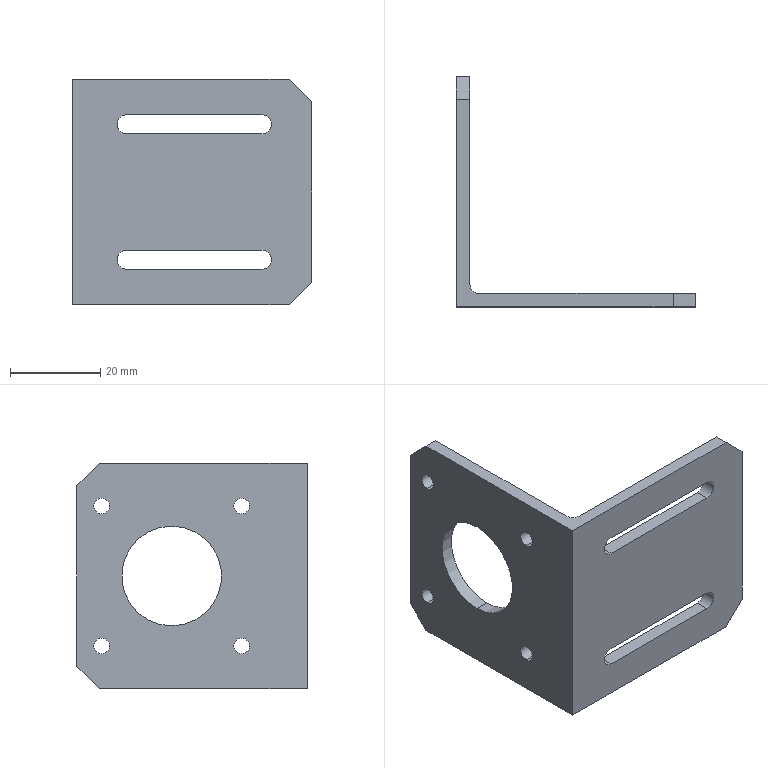Part | SolidWorks | features BaseBody 1 | 1 solid | 31 faces | box 53 x 51 x 50 mm | volume 12938 mm3 | plane 16 | cylinder 15 | commonest cylinder face diameters 3.5 x8 4.2 x4 22.1 x2 4 x1
STEP:
#1=CARTESIAN_POINT('',(3.,30.,11.05));
#2=VERTEX_POINT('',#1);
#3=CARTESIAN_POINT('',(3.,30.,-11.05));
#4=VERTEX_POINT('',#3);
#5=CARTESIAN_POINT('',(3.,30.,0.));
#6=DIRECTION('',(1.,0.,0.));
#7=DIRECTION('',(0.,0.,1.));
#8=AXIS2_PLACEMENT_3D('',#5,#6,#7);
#9=CIRCLE('',#8,11.05);
#10=EDGE_CURVE('',#2,#4,#9,.T.);
#11=ORIENTED_EDGE('',*,*,#10,.T.);
#12=CARTESIAN_POINT('',(0.,30.,-11.05));
#13=VERTEX_POINT('',#12);
#14=CARTESIAN_POINT('',(20.,30.,-11.05));
#15=DIRECTION('',(-1.,0.,0.));
#16=VECTOR('',#15,1000.);
#17=LINE('',#14,#16);
#18=EDGE_CURVE('',#4,#13,#17,.T.);
#19=ORIENTED_EDGE('',*,*,#18,.T.);
#20=CARTESIAN_POINT('',(0.,30.,11.05));
#21=VERTEX_POINT('',#20);
#22=CARTESIAN_POINT('',(0.,30.,0.));
#23=DIRECTION('',(-1.,0.,0.));
#24=DIRECTION('',(0.,0.,1.));
#25=AXIS2_PLACEMENT_3D('',#22,#23,#24);
#26=CIRCLE('',#25,11.05);
#27=EDGE_CURVE('',#13,#21,#26,.T.);
#28=ORIENTED_EDGE('',*,*,#27,.T.);
#29=CARTESIAN_POINT('',(20.,30.,11.05));
#30=DIRECTION('',(-1.,0.,0.));
#31=VECTOR('',#30,1000.);
#32=LINE('',#29,#31);
#33=EDGE_CURVE('',#2,#21,#32,.T.);
#34=ORIENTED_EDGE('',*,*,#33,.F.);
#35=EDGE_LOOP('',(#11,#19,#28,#34));
#36=FACE_OUTER_BOUND('',#35,.T.);
#37=CARTESIAN_POINT('',(20.,30.,0.));
#38=DIRECTION('',(-1.,0.,0.));
#39=DIRECTION('',(0.,0.,1.));
#40=AXIS2_PLACEMENT_3D('',#37,#38,#39);
#41=CYLINDRICAL_SURFACE('',#40,11.05);
#42=ADVANCED_FACE('',(#36),#41,.F.);
#43=CARTESIAN_POINT('',(3.,45.5,-13.75));
#44=VERTEX_POINT('',#43);
#45=CARTESIAN_POINT('',(3.,45.5,-17.25));
#46=VERTEX_POINT('',#45);
#47=CARTESIAN_POINT('',(3.,45.5,-15.5));
#48=DIRECTION('',(1.,0.,0.));
#49=DIRECTION('',(0.,0.,1.));
#50=AXIS2_PLACEMENT_3D('',#47,#48,#49);
#51=CIRCLE('',#50,1.75);
#52=EDGE_CURVE('',#44,#46,#51,.T.);
#53=ORIENTED_EDGE('',*,*,#52,.T.);
#54=CARTESIAN_POINT('',(0.,45.5,-17.25));
#55=VERTEX_POINT('',#54);
#56=CARTESIAN_POINT('',(20.,45.5,-17.25));
#57=DIRECTION('',(-1.,0.,0.));
#58=VECTOR('',#57,1000.);
#59=LINE('',#56,#58);
#60=EDGE_CURVE('',#46,#55,#59,.T.);
#61=ORIENTED_EDGE('',*,*,#60,.T.);
#62=CARTESIAN_POINT('',(0.,45.5,-13.75));
#63=VERTEX_POINT('',#62);
#64=CARTESIAN_POINT('',(0.,45.5,-15.5));
#65=DIRECTION('',(-1.,0.,0.));
#66=DIRECTION('',(0.,0.,1.));
#67=AXIS2_PLACEMENT_3D('',#64,#65,#66);
#68=CIRCLE('',#67,1.75);
#69=EDGE_CURVE('',#55,#63,#68,.T.);
#70=ORIENTED_EDGE('',*,*,#69,.T.);
#71=CARTESIAN_POINT('',(20.,45.5,-13.75));
#72=DIRECTION('',(-1.,0.,0.));
#73=VECTOR('',#72,1000.);
#74=LINE('',#71,#73);
#75=EDGE_CURVE('',#44,#63,#74,.T.);
#76=ORIENTED_EDGE('',*,*,#75,.F.);
#77=EDGE_LOOP('',(#53,#61,#70,#76));
#78=FACE_OUTER_BOUND('',#77,.T.);
#79=CARTESIAN_POINT('',(20.,45.5,-15.5));
#80=DIRECTION('',(-1.,0.,0.));
#81=DIRECTION('',(0.,0.,1.));
#82=AXIS2_PLACEMENT_3D('',#79,#80,#81);
#83=CYLINDRICAL_SURFACE('',#82,1.75);
#84=ADVANCED_FACE('',(#78),#83,.F.);
#85=CARTESIAN_POINT('',(3.,45.5,17.25));
#86=VERTEX_POINT('',#85);
#87=CARTESIAN_POINT('',(3.,45.5,13.75));
#88=VERTEX_POINT('',#87);
#89=CARTESIAN_POINT('',(3.,45.5,15.5));
#90=DIRECTION('',(1.,0.,0.));
#91=DIRECTION('',(0.,0.,1.));
#92=AXIS2_PLACEMENT_3D('',#89,#90,#91);
#93=CIRCLE('',#92,1.75);
#94=EDGE_CURVE('',#86,#88,#93,.T.);
#95=ORIENTED_EDGE('',*,*,#94,.T.);
#96=CARTESIAN_POINT('',(0.,45.5,13.75));
#97=VERTEX_POINT('',#96);
#98=CARTESIAN_POINT('',(20.,45.5,13.75));
#99=DIRECTION('',(-1.,0.,0.));
#100=VECTOR('',#99,1000.);
#101=LINE('',#98,#100);
#102=EDGE_CURVE('',#88,#97,#101,.T.);
#103=ORIENTED_EDGE('',*,*,#102,.T.);
#104=CARTESIAN_POINT('',(0.,45.5,17.25));
#105=VERTEX_POINT('',#104);
#106=CARTESIAN_POINT('',(0.,45.5,15.5));
#107=DIRECTION('',(-1.,0.,0.));
#108=DIRECTION('',(0.,0.,1.));
#109=AXIS2_PLACEMENT_3D('',#106,#107,#108);
#110=CIRCLE('',#109,1.75);
#111=EDGE_CURVE('',#97,#105,#110,.T.);
#112=ORIENTED_EDGE('',*,*,#111,.T.);
#113=CARTESIAN_POINT('',(20.,45.5,17.25));
#114=DIRECTION('',(-1.,0.,0.));
#115=VECTOR('',#114,1000.);
#116=LINE('',#113,#115);
#117=EDGE_CURVE('',#86,#105,#116,.T.);
#118=ORIENTED_EDGE('',*,*,#117,.F.);
#119=EDGE_LOOP('',(#95,#103,#112,#118));
#120=FACE_OUTER_BOUND('',#119,.T.);
#121=CARTESIAN_POINT('',(20.,45.5,15.5));
#122=DIRECTION('',(-1.,0.,0.));
#123=DIRECTION('',(0.,0.,1.));
#124=AXIS2_PLACEMENT_3D('',#121,#122,#123);
#125=CYLINDRICAL_SURFACE('',#124,1.75);
#126=ADVANCED_FACE('',(#120),#125,.F.);
#127=CARTESIAN_POINT('',(3.,14.5,-13.75));
#128=VERTEX_POINT('',#127);
#129=CARTESIAN_POINT('',(3.,14.5,-17.25));
#130=VERTEX_POINT('',#129);
#131=CARTESIAN_POINT('',(3.,14.5,-15.5));
#132=DIRECTION('',(1.,0.,0.));
#133=DIRECTION('',(0.,0.,1.));
#134=AXIS2_PLACEMENT_3D('',#131,#132,#133);
#135=CIRCLE('',#134,1.75);
#136=EDGE_CURVE('',#128,#130,#135,.T.);
#137=ORIENTED_EDGE('',*,*,#136,.T.);
#138=CARTESIAN_POINT('',(0.,14.5,-17.25));
#139=VERTEX_POINT('',#138);
#140=CARTESIAN_POINT('',(20.,14.5,-17.25));
#141=DIRECTION('',(-1.,0.,0.));
#142=VECTOR('',#141,1000.);
#143=LINE('',#140,#142);
#144=EDGE_CURVE('',#130,#139,#143,.T.);
#145=ORIENTED_EDGE('',*,*,#144,.T.);
#146=CARTESIAN_POINT('',(0.,14.5,-13.75));
#147=VERTEX_POINT('',#146);
#148=CARTESIAN_POINT('',(0.,14.5,-15.5));
#149=DIRECTION('',(-1.,0.,0.));
#150=DIRECTION('',(0.,0.,1.));
#151=AXIS2_PLACEMENT_3D('',#148,#149,#150);
#152=CIRCLE('',#151,1.75);
#153=EDGE_CURVE('',#139,#147,#152,.T.);
#154=ORIENTED_EDGE('',*,*,#153,.T.);
#155=CARTESIAN_POINT('',(20.,14.5,-13.75));
#156=DIRECTION('',(-1.,0.,0.));
#157=VECTOR('',#156,1000.);
#158=LINE('',#155,#157);
#159=EDGE_CURVE('',#128,#147,#158,.T.);
#160=ORIENTED_EDGE('',*,*,#159,.F.);
#161=EDGE_LOOP('',(#137,#145,#154,#160));
#162=FACE_OUTER_BOUND('',#161,.T.);
#163=CARTESIAN_POINT('',(20.,14.5,-15.5));
#164=DIRECTION('',(-1.,0.,0.));
#165=DIRECTION('',(0.,0.,1.));
#166=AXIS2_PLACEMENT_3D('',#163,#164,#165);
#167=CYLINDRICAL_SURFACE('',#166,1.75);
#168=ADVANCED_FACE('',(#162),#167,.F.);
#169=CARTESIAN_POINT('',(3.,14.5,17.25));
#170=VERTEX_POINT('',#169);
#171=CARTESIAN_POINT('',(3.,14.5,13.75));
#172=VERTEX_POINT('',#171);
#173=CARTESIAN_POINT('',(3.,14.5,15.5));
#174=DIRECTION('',(1.,0.,0.));
#175=DIRECTION('',(0.,0.,1.));
#176=AXIS2_PLACEMENT_3D('',#173,#174,#175);
#177=CIRCLE('',#176,1.75);
#178=EDGE_CURVE('',#170,#172,#177,.T.);
#179=ORIENTED_EDGE('',*,*,#178,.T.);
#180=CARTESIAN_POINT('',(0.,14.5,13.75));
#181=VERTEX_POINT('',#180);
#182=CARTESIAN_POINT('',(20.,14.5,13.75));
#183=DIRECTION('',(-1.,0.,0.));
#184=VECTOR('',#183,1000.);
#185=LINE('',#182,#184);
#186=EDGE_CURVE('',#172,#181,#185,.T.);
#187=ORIENTED_EDGE('',*,*,#186,.T.);
#188=CARTESIAN_POINT('',(0.,14.5,17.25));
#189=VERTEX_POINT('',#188);
#190=CARTESIAN_POINT('',(0.,14.5,15.5));
#191=DIRECTION('',(-1.,0.,0.));
#192=DIRECTION('',(0.,0.,1.));
#193=AXIS2_PLACEMENT_3D('',#190,#191,#192);
#194=CIRCLE('',#193,1.75);
#195=EDGE_CURVE('',#181,#189,#194,.T.);
#196=ORIENTED_EDGE('',*,*,#195,.T.);
#197=CARTESIAN_POINT('',(20.,14.5,17.25));
#198=DIRECTION('',(-1.,0.,0.));
#199=VECTOR('',#198,1000.);
#200=LINE('',#197,#199);
#201=EDGE_CURVE('',#170,#189,#200,.T.);
#202=ORIENTED_EDGE('',*,*,#201,.F.);
#203=EDGE_LOOP('',(#179,#187,#196,#202));
#204=FACE_OUTER_BOUND('',#203,.T.);
#205=CARTESIAN_POINT('',(20.,14.5,15.5));
#206=DIRECTION('',(-1.,0.,0.));
#207=DIRECTION('',(0.,0.,1.));
#208=AXIS2_PLACEMENT_3D('',#205,#206,#207);
#209=CYLINDRICAL_SURFACE('',#208,1.75);
#210=ADVANCED_FACE('',(#204),#209,.F.);
#211=CARTESIAN_POINT('',(53.,0.,-20.));
#212=VERTEX_POINT('',#211);
#213=CARTESIAN_POINT('',(48.,0.,-25.));
#214=VERTEX_POINT('',#213);
#215=CARTESIAN_POINT('',(53.,0.,-20.));
#216=DIRECTION('',(-0.7071,0.,-0.7071));
#217=VECTOR('',#216,1000.);
#218=LINE('',#215,#217);
#219=EDGE_CURVE('',#212,#214,#218,.T.);
#220=ORIENTED_EDGE('',*,*,#219,.F.);
#221=CARTESIAN_POINT('',(53.,0.,20.));
#222=VERTEX_POINT('',#221);
#223=CARTESIAN_POINT('',(53.,0.,25.));
#224=DIRECTION('',(0.,0.,-1.));
#225=VECTOR('',#224,1000.);
#226=LINE('',#223,#225);
#227=EDGE_CURVE('',#222,#212,#226,.T.);
#228=ORIENTED_EDGE('',*,*,#227,.F.);
#229=CARTESIAN_POINT('',(48.,0.,25.));
#230=VERTEX_POINT('',#229);
#231=CARTESIAN_POINT('',(48.,0.,25.));
#232=DIRECTION('',(0.7071,0.,-0.7071));
#233=VECTOR('',#232,1000.);
#234=LINE('',#231,#233);
#235=EDGE_CURVE('',#230,#222,#234,.T.);
#236=ORIENTED_EDGE('',*,*,#235,.F.);
#237=CARTESIAN_POINT('',(0.,0.,25.));
#238=VERTEX_POINT('',#237);
#239=CARTESIAN_POINT('',(53.,0.,25.));
#240=DIRECTION('',(1.,0.,0.));
#241=VECTOR('',#240,1000.);
#242=LINE('',#239,#241);
#243=EDGE_CURVE('',#238,#230,#242,.T.);
#244=ORIENTED_EDGE('',*,*,#243,.F.);
#245=CARTESIAN_POINT('',(0.,0.,-25.));
#246=VERTEX_POINT('',#245);
#247=CARTESIAN_POINT('',(0.,0.,25.));
#248=DIRECTION('',(0.,0.,1.));
#249=VECTOR('',#248,1000.);
#250=LINE('',#247,#249);
#251=EDGE_CURVE('',#246,#238,#250,.T.);
#252=ORIENTED_EDGE('',*,*,#251,.F.);
#253=CARTESIAN_POINT('',(53.,0.,-25.));
#254=DIRECTION('',(-1.,0.,0.));
#255=VECTOR('',#254,1000.);
#256=LINE('',#253,#255);
#257=EDGE_CURVE('',#214,#246,#256,.T.);
#258=ORIENTED_EDGE('',*,*,#257,.F.);
#259=EDGE_LOOP('',(#220,#228,#236,#244,#252,#258));
#260=FACE_OUTER_BOUND('',#259,.T.);
#261=CARTESIAN_POINT('',(12.,0.,17.1));
#262=VERTEX_POINT('',#261);
#263=CARTESIAN_POINT('',(12.,0.,12.9));
#264=VERTEX_POINT('',#263);
#265=CARTESIAN_POINT('',(12.,0.,15.));
#266=DIRECTION('',(0.,-1.,0.));
#267=DIRECTION('',(0.,0.,1.));
#268=AXIS2_PLACEMENT_3D('',#265,#266,#267);
#269=CIRCLE('',#268,2.1);
#270=EDGE_CURVE('',#262,#264,#269,.T.);
#271=ORIENTED_EDGE('',*,*,#270,.F.);
#272=CARTESIAN_POINT('',(42.,0.,17.1));
#273=VERTEX_POINT('',#272);
#274=CARTESIAN_POINT('',(53.,0.,17.1));
#275=DIRECTION('',(-1.,0.,0.));
#276=VECTOR('',#275,1000.);
#277=LINE('',#274,#276);
#278=EDGE_CURVE('',#273,#262,#277,.T.);
#279=ORIENTED_EDGE('',*,*,#278,.F.);
#280=CARTESIAN_POINT('',(42.,0.,12.9));
#281=VERTEX_POINT('',#280);
#282=CARTESIAN_POINT('',(42.,0.,15.));
#283=DIRECTION('',(0.,-1.,0.));
#284=DIRECTION('',(0.,0.,1.));
#285=AXIS2_PLACEMENT_3D('',#282,#283,#284);
#286=CIRCLE('',#285,2.1);
#287=EDGE_CURVE('',#281,#273,#286,.T.);
#288=ORIENTED_EDGE('',*,*,#287,.F.);
#289=CARTESIAN_POINT('',(53.,0.,12.9));
#290=DIRECTION('',(1.,0.,0.));
#291=VECTOR('',#290,1000.);
#292=LINE('',#289,#291);
#293=EDGE_CURVE('',#264,#281,#292,.T.);
#294=ORIENTED_EDGE('',*,*,#293,.F.);
#295=EDGE_LOOP('',(#271,#279,#288,#294));
#296=FACE_BOUND('',#295,.T.);
#297=CARTESIAN_POINT('',(12.,0.,-12.9));
#298=VERTEX_POINT('',#297);
#299=CARTESIAN_POINT('',(12.,0.,-17.1));
#300=VERTEX_POINT('',#299);
#301=CARTESIAN_POINT('',(12.,0.,-15.));
#302=DIRECTION('',(0.,-1.,0.));
#303=DIRECTION('',(0.,0.,1.));
#304=AXIS2_PLACEMENT_3D('',#301,#302,#303);
#305=CIRCLE('',#304,2.1);
#306=EDGE_CURVE('',#298,#300,#305,.T.);
#307=ORIENTED_EDGE('',*,*,#306,.F.);
#308=CARTESIAN_POINT('',(42.,0.,-12.9));
#309=VERTEX_POINT('',#308);
#310=CARTESIAN_POINT('',(53.,0.,-12.9));
#311=DIRECTION('',(-1.,0.,0.));
#312=VECTOR('',#311,1000.);
#313=LINE('',#310,#312);
#314=EDGE_CURVE('',#309,#298,#313,.T.);
#315=ORIENTED_EDGE('',*,*,#314,.F.);
#316=CARTESIAN_POINT('',(42.,0.,-17.1));
#317=VERTEX_POINT('',#316);
#318=CARTESIAN_POINT('',(42.,0.,-15.));
#319=DIRECTION('',(0.,-1.,0.));
#320=DIRECTION('',(0.,0.,1.));
#321=AXIS2_PLACEMENT_3D('',#318,#319,#320);
#322=CIRCLE('',#321,2.1);
#323=EDGE_CURVE('',#317,#309,#322,.T.);
#324=ORIENTED_EDGE('',*,*,#323,.F.);
#325=CARTESIAN_POINT('',(53.,0.,-17.1));
#326=DIRECTION('',(1.,0.,0.));
#327=VECTOR('',#326,1000.);
#328=LINE('',#325,#327);
#329=EDGE_CURVE('',#300,#317,#328,.T.);
#330=ORIENTED_EDGE('',*,*,#329,.F.);
#331=EDGE_LOOP('',(#307,#315,#324,#330));
#332=FACE_BOUND('',#331,.T.);
#333=CARTESIAN_POINT('',(53.,0.,25.));
#334=DIRECTION('',(0.,1.,0.));
#335=DIRECTION('',(0.,0.,1.));
#336=AXIS2_PLACEMENT_3D('',#333,#334,#335);
#337=PLANE('',#336);
#338=ADVANCED_FACE('',(#260,#296,#332),#337,.F.);
#339=CARTESIAN_POINT('',(3.,46.,-25.));
#340=VERTEX_POINT('',#339);
#341=CARTESIAN_POINT('',(3.,5.,-25.));
#342=VERTEX_POINT('',#341);
#343=CARTESIAN_POINT('',(3.,0.,-25.));
#344=DIRECTION('',(0.,-1.,0.));
#345=VECTOR('',#344,1000.);
#346=LINE('',#343,#345);
#347=EDGE_CURVE('',#340,#342,#346,.T.);
#348=ORIENTED_EDGE('',*,*,#347,.T.);
#349=CARTESIAN_POINT('',(5.,3.,-25.));
#350=VERTEX_POINT('',#349);
#351=CARTESIAN_POINT('',(5.,5.,-25.));
#352=DIRECTION('',(0.,0.,1.));
#353=DIRECTION('',(1.,0.,0.));
#354=AXIS2_PLACEMENT_3D('',#351,#352,#353);
#355=CIRCLE('',#354,2.);
#356=EDGE_CURVE('',#342,#350,#355,.T.);
#357=ORIENTED_EDGE('',*,*,#356,.T.);
#358=CARTESIAN_POINT('',(48.,3.,-25.));
#359=VERTEX_POINT('',#358);
#360=CARTESIAN_POINT('',(0.,3.,-25.));
#361=DIRECTION('',(1.,0.,0.));
#362=VECTOR('',#361,1000.);
#363=LINE('',#360,#362);
#364=EDGE_CURVE('',#350,#359,#363,.T.);
#365=ORIENTED_EDGE('',*,*,#364,.T.);
#366=CARTESIAN_POINT('',(48.,0.,-25.));
#367=DIRECTION('',(0.,-1.,0.));
#368=VECTOR('',#367,1000.);
#369=LINE('',#366,#368);
#370=EDGE_CURVE('',#359,#214,#369,.T.);
#371=ORIENTED_EDGE('',*,*,#370,.T.);
#372=ORIENTED_EDGE('',*,*,#257,.T.);
#373=CARTESIAN_POINT('',(0.,46.,-25.));
#374=VERTEX_POINT('',#373);
#375=CARTESIAN_POINT('',(0.,0.,-25.));
#376=DIRECTION('',(0.,1.,0.));
#377=VECTOR('',#376,1000.);
#378=LINE('',#375,#377);
#379=EDGE_CURVE('',#246,#374,#378,.T.);
#380=ORIENTED_EDGE('',*,*,#379,.T.);
#381=CARTESIAN_POINT('',(0.,46.,-25.));
#382=DIRECTION('',(1.,0.,0.));
#383=VECTOR('',#382,1000.);
#384=LINE('',#381,#383);
#385=EDGE_CURVE('',#374,#340,#384,.T.);
#386=ORIENTED_EDGE('',*,*,#385,.T.);
#387=EDGE_LOOP('',(#348,#357,#365,#371,#372,#380,#386));
#388=FACE_OUTER_BOUND('',#387,.T.);
#389=CARTESIAN_POINT('',(0.,0.,-25.));
#390=DIRECTION('',(0.,0.,-1.));
#391=DIRECTION('',(-1.,0.,0.));
#392=AXIS2_PLACEMENT_3D('',#389,#390,#391);
#393=PLANE('',#392);
#394=ADVANCED_FACE('',(#388),#393,.T.);
#395=CARTESIAN_POINT('',(53.,3.,-20.));
#396=VERTEX_POINT('',#395);
#397=CARTESIAN_POINT('',(53.,3.,-20.));
#398=DIRECTION('',(0.7071,0.,0.7071));
#399=VECTOR('',#398,1000.);
#400=LINE('',#397,#399);
#401=EDGE_CURVE('',#359,#396,#400,.T.);
#402=ORIENTED_EDGE('',*,*,#401,.T.);
#403=CARTESIAN_POINT('',(53.,3.,-20.));
#404=DIRECTION('',(0.,-1.,0.));
#405=VECTOR('',#404,1000.);
#406=LINE('',#403,#405);
#407=EDGE_CURVE('',#396,#212,#406,.T.);
#408=ORIENTED_EDGE('',*,*,#407,.T.);
#409=ORIENTED_EDGE('',*,*,#219,.T.);
#410=ORIENTED_EDGE('',*,*,#370,.F.);
#411=EDGE_LOOP('',(#402,#408,#409,#410));
#412=FACE_OUTER_BOUND('',#411,.T.);
#413=CARTESIAN_POINT('',(53.,3.,-20.));
#414=DIRECTION('',(0.7071,0.,-0.7071));
#415=DIRECTION('',(-0.7071,0.,-0.7071));
#416=AXIS2_PLACEMENT_3D('',#413,#414,#415);
#417=PLANE('',#416);
#418=ADVANCED_FACE('',(#412),#417,.T.);
#419=ORIENTED_EDGE('',*,*,#407,.F.);
#420=CARTESIAN_POINT('',(53.,3.,20.));
#421=VERTEX_POINT('',#420);
#422=CARTESIAN_POINT('',(53.,3.,25.));
#423=DIRECTION('',(0.,0.,-1.));
#424=VECTOR('',#423,1000.);
#425=LINE('',#422,#424);
#426=EDGE_CURVE('',#421,#396,#425,.T.);
#427=ORIENTED_EDGE('',*,*,#426,.F.);
#428=CARTESIAN_POINT('',(53.,3.,20.));
#429=DIRECTION('',(0.,1.,0.));
#430=VECTOR('',#429,1000.);
#431=LINE('',#428,#430);
#432=EDGE_CURVE('',#222,#421,#431,.T.);
#433=ORIENTED_EDGE('',*,*,#432,.F.);
#434=ORIENTED_EDGE('',*,*,#227,.T.);
#435=EDGE_LOOP('',(#419,#427,#433,#434));
#436=FACE_OUTER_BOUND('',#435,.T.);
#437=CARTESIAN_POINT('',(53.,3.,25.));
#438=DIRECTION('',(-1.,0.,0.));
#439=DIRECTION('',(0.,0.,1.));
#440=AXIS2_PLACEMENT_3D('',#437,#438,#439);
#441=PLANE('',#440);
#442=ADVANCED_FACE('',(#436),#441,.F.);
#443=ORIENTED_EDGE('',*,*,#432,.T.);
#444=CARTESIAN_POINT('',(48.,3.,25.));
#445=VERTEX_POINT('',#444);
#446=CARTESIAN_POINT('',(48.,3.,25.));
#447=DIRECTION('',(0.7071,0.,-0.7071));
#448=VECTOR('',#447,1000.);
#449=LINE('',#446,#448);
#450=EDGE_CURVE('',#445,#421,#449,.T.);
#451=ORIENTED_EDGE('',*,*,#450,.F.);
#452=CARTESIAN_POINT('',(48.,0.,25.));
#453=DIRECTION('',(0.,1.,0.));
#454=VECTOR('',#453,1000.);
#455=LINE('',#452,#454);
#456=EDGE_CURVE('',#230,#445,#455,.T.);
#457=ORIENTED_EDGE('',*,*,#456,.F.);
#458=ORIENTED_EDGE('',*,*,#235,.T.);
#459=EDGE_LOOP('',(#443,#451,#457,#458));
#460=FACE_OUTER_BOUND('',#459,.T.);
#461=CARTESIAN_POINT('',(48.,0.,25.));
#462=DIRECTION('',(-0.7071,0.,-0.7071));
#463=DIRECTION('',(-0.7071,0.,0.7071));
#464=AXIS2_PLACEMENT_3D('',#461,#462,#463);
#465=PLANE('',#464);
#466=ADVANCED_FACE('',(#460),#465,.F.);
#467=ORIENTED_EDGE('',*,*,#456,.T.);
#468=CARTESIAN_POINT('',(5.,3.,25.));
#469=VERTEX_POINT('',#468);
#470=CARTESIAN_POINT('',(0.,3.,25.));
#471=DIRECTION('',(1.,0.,0.));
#472=VECTOR('',#471,1000.);
#473=LINE('',#470,#472);
#474=EDGE_CURVE('',#469,#445,#473,.T.);
#475=ORIENTED_EDGE('',*,*,#474,.F.);
#476=CARTESIAN_POINT('',(3.,5.,25.));
#477=VERTEX_POINT('',#476);
#478=CARTESIAN_POINT('',(5.,5.,25.));
#479=DIRECTION('',(0.,0.,1.));
#480=DIRECTION('',(1.,0.,0.));
#481=AXIS2_PLACEMENT_3D('',#478,#479,#480);
#482=CIRCLE('',#481,2.);
#483=EDGE_CURVE('',#477,#469,#482,.T.);
#484=ORIENTED_EDGE('',*,*,#483,.F.);
#485=CARTESIAN_POINT('',(3.,46.,25.));
#486=VERTEX_POINT('',#485);
#487=CARTESIAN_POINT('',(3.,0.,25.));
#488=DIRECTION('',(0.,-1.,0.));
#489=VECTOR('',#488,1000.);
#490=LINE('',#487,#489);
#491=EDGE_CURVE('',#486,#477,#490,.T.);
#492=ORIENTED_EDGE('',*,*,#491,.F.);
#493=CARTESIAN_POINT('',(0.,46.,25.));
#494=VERTEX_POINT('',#493);
#495=CARTESIAN_POINT('',(0.,46.,25.));
#496=DIRECTION('',(1.,0.,0.));
#497=VECTOR('',#496,1000.);
#498=LINE('',#495,#497);
#499=EDGE_CURVE('',#494,#486,#498,.T.);
#500=ORIENTED_EDGE('',*,*,#499,.F.);
#501=CARTESIAN_POINT('',(0.,0.,25.));
#502=DIRECTION('',(0.,1.,0.));
#503=VECTOR('',#502,1000.);
#504=LINE('',#501,#503);
#505=EDGE_CURVE('',#238,#494,#504,.T.);
#506=ORIENTED_EDGE('',*,*,#505,.F.);
#507=ORIENTED_EDGE('',*,*,#243,.T.);
#508=EDGE_LOOP('',(#467,#475,#484,#492,#500,#506,#507));
#509=FACE_OUTER_BOUND('',#508,.T.);
#510=CARTESIAN_POINT('',(0.,0.,25.));
#511=DIRECTION('',(0.,0.,-1.));
#512=DIRECTION('',(-1.,0.,0.));
#513=AXIS2_PLACEMENT_3D('',#510,#511,#512);
#514=PLANE('',#513);
#515=ADVANCED_FACE('',(#509),#514,.F.);
#516=CARTESIAN_POINT('',(0.,51.,20.));
#517=VERTEX_POINT('',#516);
#518=CARTESIAN_POINT('',(0.,51.,20.));
#519=DIRECTION('',(0.,-0.7071,0.7071));
#520=VECTOR('',#519,1000.);
#521=LINE('',#518,#520);
#522=EDGE_CURVE('',#517,#494,#521,.T.);
#523=ORIENTED_EDGE('',*,*,#522,.F.);
#524=CARTESIAN_POINT('',(0.,51.,-20.));
#525=VERTEX_POINT('',#524);
#526=CARTESIAN_POINT('',(0.,51.,25.));
#527=DIRECTION('',(0.,0.,1.));
#528=VECTOR('',#527,1000.);
#529=LINE('',#526,#528);
#530=EDGE_CURVE('',#525,#517,#529,.T.);
#531=ORIENTED_EDGE('',*,*,#530,.F.);
#532=CARTESIAN_POINT('',(0.,46.,-25.));
#533=DIRECTION('',(0.,0.7071,0.7071));
#534=VECTOR('',#533,1000.);
#535=LINE('',#532,#534);
#536=EDGE_CURVE('',#374,#525,#535,.T.);
#537=ORIENTED_EDGE('',*,*,#536,.F.);
#538=ORIENTED_EDGE('',*,*,#379,.F.);
#539=ORIENTED_EDGE('',*,*,#251,.T.);
#540=ORIENTED_EDGE('',*,*,#505,.T.);
#541=EDGE_LOOP('',(#523,#531,#537,#538,#539,#540));
#542=FACE_OUTER_BOUND('',#541,.T.);
#543=CARTESIAN_POINT('',(0.,30.,0.));
#544=DIRECTION('',(-1.,0.,0.));
#545=DIRECTION('',(0.,0.,1.));
#546=AXIS2_PLACEMENT_3D('',#543,#544,#545);
#547=CIRCLE('',#546,11.05);
#548=EDGE_CURVE('',#21,#13,#547,.T.);
#549=ORIENTED_EDGE('',*,*,#548,.F.);
#550=ORIENTED_EDGE('',*,*,#27,.F.);
#551=EDGE_LOOP('',(#549,#550));
#552=FACE_BOUND('',#551,.T.);
#553=CARTESIAN_POINT('',(0.,45.5,-15.5));
#554=DIRECTION('',(-1.,0.,0.));
#555=DIRECTION('',(0.,0.,1.));
#556=AXIS2_PLACEMENT_3D('',#553,#554,#555);
#557=CIRCLE('',#556,1.75);
#558=EDGE_CURVE('',#63,#55,#557,.T.);
#559=ORIENTED_EDGE('',*,*,#558,.F.);
#560=ORIENTED_EDGE('',*,*,#69,.F.);
#561=EDGE_LOOP('',(#559,#560));
#562=FACE_BOUND('',#561,.T.);
#563=CARTESIAN_POINT('',(0.,45.5,15.5));
#564=DIRECTION('',(-1.,0.,0.));
#565=DIRECTION('',(0.,0.,1.));
#566=AXIS2_PLACEMENT_3D('',#563,#564,#565);
#567=CIRCLE('',#566,1.75);
#568=EDGE_CURVE('',#105,#97,#567,.T.);
#569=ORIENTED_EDGE('',*,*,#568,.F.);
#570=ORIENTED_EDGE('',*,*,#111,.F.);
#571=EDGE_LOOP('',(#569,#570));
#572=FACE_BOUND('',#571,.T.);
#573=CARTESIAN_POINT('',(0.,14.5,-15.5));
#574=DIRECTION('',(-1.,0.,0.));
#575=DIRECTION('',(0.,0.,1.));
#576=AXIS2_PLACEMENT_3D('',#573,#574,#575);
#577=CIRCLE('',#576,1.75);
#578=EDGE_CURVE('',#147,#139,#577,.T.);
#579=ORIENTED_EDGE('',*,*,#578,.F.);
#580=ORIENTED_EDGE('',*,*,#153,.F.);
#581=EDGE_LOOP('',(#579,#580));
#582=FACE_BOUND('',#581,.T.);
#583=CARTESIAN_POINT('',(0.,14.5,15.5));
#584=DIRECTION('',(-1.,0.,0.));
#585=DIRECTION('',(0.,0.,1.));
#586=AXIS2_PLACEMENT_3D('',#583,#584,#585);
#587=CIRCLE('',#586,1.75);
#588=EDGE_CURVE('',#189,#181,#587,.T.);
#589=ORIENTED_EDGE('',*,*,#588,.F.);
#590=ORIENTED_EDGE('',*,*,#195,.F.);
#591=EDGE_LOOP('',(#589,#590));
#592=FACE_BOUND('',#591,.T.);
#593=CARTESIAN_POINT('',(0.,0.,25.));
#594=DIRECTION('',(1.,0.,0.));
#595=DIRECTION('',(0.,0.,-1.));
#596=AXIS2_PLACEMENT_3D('',#593,#594,#595);
#597=PLANE('',#596);
#598=ADVANCED_FACE('',(#542,#552,#562,#572,#582,#592),#597,.F.);
#599=CARTESIAN_POINT('',(12.,3.,12.9));
#600=VERTEX_POINT('',#599);
#601=CARTESIAN_POINT('',(42.,3.,12.9));
#602=VERTEX_POINT('',#601);
#603=CARTESIAN_POINT('',(12.,3.,12.9));
#604=DIRECTION('',(1.,0.,0.));
#605=VECTOR('',#604,1000.);
#606=LINE('',#603,#605);
#607=EDGE_CURVE('',#600,#602,#606,.T.);
#608=ORIENTED_EDGE('',*,*,#607,.F.);
#609=CARTESIAN_POINT('',(12.,-17.,12.9));
#610=DIRECTION('',(0.,1.,0.));
#611=VECTOR('',#610,1000.);
#612=LINE('',#609,#611);
#613=EDGE_CURVE('',#264,#600,#612,.T.);
#614=ORIENTED_EDGE('',*,*,#613,.F.);
#615=ORIENTED_EDGE('',*,*,#293,.T.);
#616=CARTESIAN_POINT('',(42.,-17.,12.9));
#617=DIRECTION('',(0.,-1.,0.));
#618=VECTOR('',#617,1000.);
#619=LINE('',#616,#618);
#620=EDGE_CURVE('',#602,#281,#619,.T.);
#621=ORIENTED_EDGE('',*,*,#620,.F.);
#622=EDGE_LOOP('',(#608,#614,#615,#621));
#623=FACE_OUTER_BOUND('',#622,.T.);
#624=CARTESIAN_POINT('',(12.,-17.,12.9));
#625=DIRECTION('',(0.,0.,-1.));
#626=DIRECTION('',(-1.,0.,0.));
#627=AXIS2_PLACEMENT_3D('',#624,#625,#626);
#628=PLANE('',#627);
#629=ADVANCED_FACE('',(#623),#628,.F.);
#630=CARTESIAN_POINT('',(12.,3.,17.1));
#631=VERTEX_POINT('',#630);
#632=CARTESIAN_POINT('',(12.,3.,15.));
#633=DIRECTION('',(0.,-1.,0.));
#634=DIRECTION('',(0.,0.,1.));
#635=AXIS2_PLACEMENT_3D('',#632,#633,#634);
#636=CIRCLE('',#635,2.1);
#637=EDGE_CURVE('',#631,#600,#636,.T.);
#638=ORIENTED_EDGE('',*,*,#637,.F.);
#639=CARTESIAN_POINT('',(12.,-17.,17.1));
#640=DIRECTION('',(0.,1.,0.));
#641=VECTOR('',#640,1000.);
#642=LINE('',#639,#641);
#643=EDGE_CURVE('',#262,#631,#642,.T.);
#644=ORIENTED_EDGE('',*,*,#643,.F.);
#645=ORIENTED_EDGE('',*,*,#270,.T.);
#646=ORIENTED_EDGE('',*,*,#613,.T.);
#647=EDGE_LOOP('',(#638,#644,#645,#646));
#648=FACE_OUTER_BOUND('',#647,.T.);
#649=CARTESIAN_POINT('',(12.,-17.,15.));
#650=DIRECTION('',(0.,1.,0.));
#651=DIRECTION('',(0.,0.,1.));
#652=AXIS2_PLACEMENT_3D('',#649,#650,#651);
#653=CYLINDRICAL_SURFACE('',#652,2.1);
#654=ADVANCED_FACE('',(#648),#653,.F.);
#655=CARTESIAN_POINT('',(42.,3.,17.1));
#656=VERTEX_POINT('',#655);
#657=CARTESIAN_POINT('',(12.,3.,17.1));
#658=DIRECTION('',(-1.,0.,0.));
#659=VECTOR('',#658,1000.);
#660=LINE('',#657,#659);
#661=EDGE_CURVE('',#656,#631,#660,.T.);
#662=ORIENTED_EDGE('',*,*,#661,.F.);
#663=CARTESIAN_POINT('',(42.,-17.,17.1));
#664=DIRECTION('',(0.,1.,0.));
#665=VECTOR('',#664,1000.);
#666=LINE('',#663,#665);
#667=EDGE_CURVE('',#273,#656,#666,.T.);
#668=ORIENTED_EDGE('',*,*,#667,.F.);
#669=ORIENTED_EDGE('',*,*,#278,.T.);
#670=ORIENTED_EDGE('',*,*,#643,.T.);
#671=EDGE_LOOP('',(#662,#668,#669,#670));
#672=FACE_OUTER_BOUND('',#671,.T.);
#673=CARTESIAN_POINT('',(12.,-17.,17.1));
#674=DIRECTION('',(0.,0.,1.));
#675=DIRECTION('',(1.,0.,0.));
#676=AXIS2_PLACEMENT_3D('',#673,#674,#675);
#677=PLANE('',#676);
#678=ADVANCED_FACE('',(#672),#677,.F.);
#679=CARTESIAN_POINT('',(42.,3.,15.));
#680=DIRECTION('',(0.,-1.,0.));
#681=DIRECTION('',(0.,0.,1.));
#682=AXIS2_PLACEMENT_3D('',#679,#680,#681);
#683=CIRCLE('',#682,2.1);
#684=EDGE_CURVE('',#602,#656,#683,.T.);
#685=ORIENTED_EDGE('',*,*,#684,.F.);
#686=ORIENTED_EDGE('',*,*,#620,.T.);
#687=ORIENTED_EDGE('',*,*,#287,.T.);
#688=ORIENTED_EDGE('',*,*,#667,.T.);
#689=EDGE_LOOP('',(#685,#686,#687,#688));
#690=FACE_OUTER_BOUND('',#689,.T.);
#691=CARTESIAN_POINT('',(42.,-17.,15.));
#692=DIRECTION('',(0.,1.,0.));
#693=DIRECTION('',(0.,0.,1.));
#694=AXIS2_PLACEMENT_3D('',#691,#692,#693);
#695=CYLINDRICAL_SURFACE('',#694,2.1);
#696=ADVANCED_FACE('',(#690),#695,.F.);
#697=CARTESIAN_POINT('',(12.,3.,-17.1));
#698=VERTEX_POINT('',#697);
#699=CARTESIAN_POINT('',(42.,3.,-17.1));
#700=VERTEX_POINT('',#699);
#701=CARTESIAN_POINT('',(12.,3.,-17.1));
#702=DIRECTION('',(1.,0.,0.));
#703=VECTOR('',#702,1000.);
#704=LINE('',#701,#703);
#705=EDGE_CURVE('',#698,#700,#704,.T.);
#706=ORIENTED_EDGE('',*,*,#705,.F.);
#707=CARTESIAN_POINT('',(12.,-17.,-17.1));
#708=DIRECTION('',(0.,1.,0.));
#709=VECTOR('',#708,1000.);
#710=LINE('',#707,#709);
#711=EDGE_CURVE('',#300,#698,#710,.T.);
#712=ORIENTED_EDGE('',*,*,#711,.F.);
#713=ORIENTED_EDGE('',*,*,#329,.T.);
#714=CARTESIAN_POINT('',(42.,-17.,-17.1));
#715=DIRECTION('',(0.,-1.,0.));
#716=VECTOR('',#715,1000.);
#717=LINE('',#714,#716);
#718=EDGE_CURVE('',#700,#317,#717,.T.);
#719=ORIENTED_EDGE('',*,*,#718,.F.);
#720=EDGE_LOOP('',(#706,#712,#713,#719));
#721=FACE_OUTER_BOUND('',#720,.T.);
#722=CARTESIAN_POINT('',(12.,-17.,-17.1));
#723=DIRECTION('',(0.,0.,-1.));
#724=DIRECTION('',(-1.,0.,0.));
#725=AXIS2_PLACEMENT_3D('',#722,#723,#724);
#726=PLANE('',#725);
#727=ADVANCED_FACE('',(#721),#726,.F.);
#728=CARTESIAN_POINT('',(12.,3.,-12.9));
#729=VERTEX_POINT('',#728);
#730=CARTESIAN_POINT('',(12.,3.,-15.));
#731=DIRECTION('',(0.,-1.,0.));
#732=DIRECTION('',(0.,0.,1.));
#733=AXIS2_PLACEMENT_3D('',#730,#731,#732);
#734=CIRCLE('',#733,2.1);
#735=EDGE_CURVE('',#729,#698,#734,.T.);
#736=ORIENTED_EDGE('',*,*,#735,.F.);
#737=CARTESIAN_POINT('',(12.,-17.,-12.9));
#738=DIRECTION('',(0.,1.,0.));
#739=VECTOR('',#738,1000.);
#740=LINE('',#737,#739);
#741=EDGE_CURVE('',#298,#729,#740,.T.);
#742=ORIENTED_EDGE('',*,*,#741,.F.);
#743=ORIENTED_EDGE('',*,*,#306,.T.);
#744=ORIENTED_EDGE('',*,*,#711,.T.);
#745=EDGE_LOOP('',(#736,#742,#743,#744));
#746=FACE_OUTER_BOUND('',#745,.T.);
#747=CARTESIAN_POINT('',(12.,-17.,-15.));
#748=DIRECTION('',(0.,1.,0.));
#749=DIRECTION('',(0.,0.,1.));
#750=AXIS2_PLACEMENT_3D('',#747,#748,#749);
#751=CYLINDRICAL_SURFACE('',#750,2.1);
#752=ADVANCED_FACE('',(#746),#751,.F.);
#753=CARTESIAN_POINT('',(42.,3.,-12.9));
#754=VERTEX_POINT('',#753);
#755=CARTESIAN_POINT('',(12.,3.,-12.9));
#756=DIRECTION('',(-1.,0.,0.));
#757=VECTOR('',#756,1000.);
#758=LINE('',#755,#757);
#759=EDGE_CURVE('',#754,#729,#758,.T.);
#760=ORIENTED_EDGE('',*,*,#759,.F.);
#761=CARTESIAN_POINT('',(42.,-17.,-12.9));
#762=DIRECTION('',(0.,1.,0.));
#763=VECTOR('',#762,1000.);
#764=LINE('',#761,#763);
#765=EDGE_CURVE('',#309,#754,#764,.T.);
#766=ORIENTED_EDGE('',*,*,#765,.F.);
#767=ORIENTED_EDGE('',*,*,#314,.T.);
#768=ORIENTED_EDGE('',*,*,#741,.T.);
#769=EDGE_LOOP('',(#760,#766,#767,#768));
#770=FACE_OUTER_BOUND('',#769,.T.);
#771=CARTESIAN_POINT('',(12.,-17.,-12.9));
#772=DIRECTION('',(0.,0.,1.));
#773=DIRECTION('',(1.,0.,0.));
#774=AXIS2_PLACEMENT_3D('',#771,#772,#773);
#775=PLANE('',#774);
#776=ADVANCED_FACE('',(#770),#775,.F.);
#777=CARTESIAN_POINT('',(42.,3.,-15.));
#778=DIRECTION('',(0.,-1.,0.));
#779=DIRECTION('',(0.,0.,1.));
#780=AXIS2_PLACEMENT_3D('',#777,#778,#779);
#781=CIRCLE('',#780,2.1);
#782=EDGE_CURVE('',#700,#754,#781,.T.);
#783=ORIENTED_EDGE('',*,*,#782,.F.);
#784=ORIENTED_EDGE('',*,*,#718,.T.);
#785=ORIENTED_EDGE('',*,*,#323,.T.);
#786=ORIENTED_EDGE('',*,*,#765,.T.);
#787=EDGE_LOOP('',(#783,#784,#785,#786));
#788=FACE_OUTER_BOUND('',#787,.T.);
#789=CARTESIAN_POINT('',(42.,-17.,-15.));
#790=DIRECTION('',(0.,1.,0.));
#791=DIRECTION('',(0.,0.,1.));
#792=AXIS2_PLACEMENT_3D('',#789,#790,#791);
#793=CYLINDRICAL_SURFACE('',#792,2.1);
#794=ADVANCED_FACE('',(#788),#793,.F.);
#795=CARTESIAN_POINT('',(5.,3.,25.));
#796=DIRECTION('',(0.,0.,1.));
#797=VECTOR('',#796,1000.);
#798=LINE('',#795,#797);
#799=EDGE_CURVE('',#350,#469,#798,.T.);
#800=ORIENTED_EDGE('',*,*,#799,.F.);
#801=ORIENTED_EDGE('',*,*,#356,.F.);
#802=CARTESIAN_POINT('',(3.,5.,25.));
#803=DIRECTION('',(0.,0.,-1.));
#804=VECTOR('',#803,1000.);
#805=LINE('',#802,#804);
#806=EDGE_CURVE('',#477,#342,#805,.T.);
#807=ORIENTED_EDGE('',*,*,#806,.F.);
#808=ORIENTED_EDGE('',*,*,#483,.T.);
#809=EDGE_LOOP('',(#800,#801,#807,#808));
#810=FACE_OUTER_BOUND('',#809,.T.);
#811=CARTESIAN_POINT('',(5.,5.,25.));
#812=DIRECTION('',(0.,0.,1.));
#813=DIRECTION('',(1.,0.,0.));
#814=AXIS2_PLACEMENT_3D('',#811,#812,#813);
#815=CYLINDRICAL_SURFACE('',#814,2.);
#816=ADVANCED_FACE('',(#810),#815,.F.);
#817=ORIENTED_EDGE('',*,*,#806,.T.);
#818=ORIENTED_EDGE('',*,*,#347,.F.);
#819=CARTESIAN_POINT('',(3.,51.,-20.));
#820=VERTEX_POINT('',#819);
#821=CARTESIAN_POINT('',(3.,51.,-20.));
#822=DIRECTION('',(0.,-0.7071,-0.7071));
#823=VECTOR('',#822,1000.);
#824=LINE('',#821,#823);
#825=EDGE_CURVE('',#820,#340,#824,.T.);
#826=ORIENTED_EDGE('',*,*,#825,.F.);
#827=CARTESIAN_POINT('',(3.,51.,20.));
#828=VERTEX_POINT('',#827);
#829=CARTESIAN_POINT('',(3.,51.,25.));
#830=DIRECTION('',(0.,0.,-1.));
#831=VECTOR('',#830,1000.);
#832=LINE('',#829,#831);
#833=EDGE_CURVE('',#828,#820,#832,.T.);
#834=ORIENTED_EDGE('',*,*,#833,.F.);
#835=CARTESIAN_POINT('',(3.,46.,25.));
#836=DIRECTION('',(0.,0.7071,-0.7071));
#837=VECTOR('',#836,1000.);
#838=LINE('',#835,#837);
#839=EDGE_CURVE('',#486,#828,#838,.T.);
#840=ORIENTED_EDGE('',*,*,#839,.F.);
#841=ORIENTED_EDGE('',*,*,#491,.T.);
#842=EDGE_LOOP('',(#817,#818,#826,#834,#840,#841));
#843=FACE_OUTER_BOUND('',#842,.T.);
#844=ORIENTED_EDGE('',*,*,#10,.F.);
#845=CARTESIAN_POINT('',(3.,30.,0.));
#846=DIRECTION('',(1.,0.,0.));
#847=DIRECTION('',(0.,0.,1.));
#848=AXIS2_PLACEMENT_3D('',#845,#846,#847);
#849=CIRCLE('',#848,11.05);
#850=EDGE_CURVE('',#4,#2,#849,.T.);
#851=ORIENTED_EDGE('',*,*,#850,.F.);
#852=EDGE_LOOP('',(#844,#851));
#853=FACE_BOUND('',#852,.T.);
#854=ORIENTED_EDGE('',*,*,#52,.F.);
#855=CARTESIAN_POINT('',(3.,45.5,-15.5));
#856=DIRECTION('',(1.,0.,0.));
#857=DIRECTION('',(0.,0.,1.));
#858=AXIS2_PLACEMENT_3D('',#855,#856,#857);
#859=CIRCLE('',#858,1.75);
#860=EDGE_CURVE('',#46,#44,#859,.T.);
#861=ORIENTED_EDGE('',*,*,#860,.F.);
#862=EDGE_LOOP('',(#854,#861));
#863=FACE_BOUND('',#862,.T.);
#864=ORIENTED_EDGE('',*,*,#94,.F.);
#865=CARTESIAN_POINT('',(3.,45.5,15.5));
#866=DIRECTION('',(1.,0.,0.));
#867=DIRECTION('',(0.,0.,1.));
#868=AXIS2_PLACEMENT_3D('',#865,#866,#867);
#869=CIRCLE('',#868,1.75);
#870=EDGE_CURVE('',#88,#86,#869,.T.);
#871=ORIENTED_EDGE('',*,*,#870,.F.);
#872=EDGE_LOOP('',(#864,#871));
#873=FACE_BOUND('',#872,.T.);
#874=ORIENTED_EDGE('',*,*,#136,.F.);
#875=CARTESIAN_POINT('',(3.,14.5,-15.5));
#876=DIRECTION('',(1.,0.,0.));
#877=DIRECTION('',(0.,0.,1.));
#878=AXIS2_PLACEMENT_3D('',#875,#876,#877);
#879=CIRCLE('',#878,1.75);
#880=EDGE_CURVE('',#130,#128,#879,.T.);
#881=ORIENTED_EDGE('',*,*,#880,.F.);
#882=EDGE_LOOP('',(#874,#881));
#883=FACE_BOUND('',#882,.T.);
#884=ORIENTED_EDGE('',*,*,#178,.F.);
#885=CARTESIAN_POINT('',(3.,14.5,15.5));
#886=DIRECTION('',(1.,0.,0.));
#887=DIRECTION('',(0.,0.,1.));
#888=AXIS2_PLACEMENT_3D('',#885,#886,#887);
#889=CIRCLE('',#888,1.75);
#890=EDGE_CURVE('',#172,#170,#889,.T.);
#891=ORIENTED_EDGE('',*,*,#890,.F.);
#892=EDGE_LOOP('',(#884,#891));
#893=FACE_BOUND('',#892,.T.);
#894=CARTESIAN_POINT('',(3.,51.,25.));
#895=DIRECTION('',(-1.,0.,0.));
#896=DIRECTION('',(0.,0.,1.));
#897=AXIS2_PLACEMENT_3D('',#894,#895,#896);
#898=PLANE('',#897);
#899=ADVANCED_FACE('',(#843,#853,#863,#873,#883,#893),#898,.F.);
#900=ORIENTED_EDGE('',*,*,#536,.T.);
#901=CARTESIAN_POINT('',(0.,51.,-20.));
#902=DIRECTION('',(1.,0.,0.));
#903=VECTOR('',#902,1000.);
#904=LINE('',#901,#903);
#905=EDGE_CURVE('',#525,#820,#904,.T.);
#906=ORIENTED_EDGE('',*,*,#905,.T.);
#907=ORIENTED_EDGE('',*,*,#825,.T.);
#908=ORIENTED_EDGE('',*,*,#385,.F.);
#909=EDGE_LOOP('',(#900,#906,#907,#908));
#910=FACE_OUTER_BOUND('',#909,.T.);
#911=CARTESIAN_POINT('',(0.,51.,-20.));
#912=DIRECTION('',(0.,0.7071,-0.7071));
#913=DIRECTION('',(0.,0.7071,0.7071));
#914=AXIS2_PLACEMENT_3D('',#911,#912,#913);
#915=PLANE('',#914);
#916=ADVANCED_FACE('',(#910),#915,.T.);
#917=ORIENTED_EDGE('',*,*,#799,.T.);
#918=ORIENTED_EDGE('',*,*,#474,.T.);
#919=ORIENTED_EDGE('',*,*,#450,.T.);
#920=ORIENTED_EDGE('',*,*,#426,.T.);
#921=ORIENTED_EDGE('',*,*,#401,.F.);
#922=ORIENTED_EDGE('',*,*,#364,.F.);
#923=EDGE_LOOP('',(#917,#918,#919,#920,#921,#922));
#924=FACE_OUTER_BOUND('',#923,.T.);
#925=ORIENTED_EDGE('',*,*,#637,.T.);
#926=ORIENTED_EDGE('',*,*,#607,.T.);
#927=ORIENTED_EDGE('',*,*,#684,.T.);
#928=ORIENTED_EDGE('',*,*,#661,.T.);
#929=EDGE_LOOP('',(#925,#926,#927,#928));
#930=FACE_BOUND('',#929,.T.);
#931=ORIENTED_EDGE('',*,*,#735,.T.);
#932=ORIENTED_EDGE('',*,*,#705,.T.);
#933=ORIENTED_EDGE('',*,*,#782,.T.);
#934=ORIENTED_EDGE('',*,*,#759,.T.);
#935=EDGE_LOOP('',(#931,#932,#933,#934));
#936=FACE_BOUND('',#935,.T.);
#937=CARTESIAN_POINT('',(3.,3.,25.));
#938=DIRECTION('',(0.,-1.,0.));
#939=DIRECTION('',(0.,0.,-1.));
#940=AXIS2_PLACEMENT_3D('',#937,#938,#939);
#941=PLANE('',#940);
#942=ADVANCED_FACE('',(#924,#930,#936),#941,.F.);
#943=CARTESIAN_POINT('',(0.,51.,20.));
#944=DIRECTION('',(1.,0.,0.));
#945=VECTOR('',#944,1000.);
#946=LINE('',#943,#945);
#947=EDGE_CURVE('',#517,#828,#946,.T.);
#948=ORIENTED_EDGE('',*,*,#947,.F.);
#949=ORIENTED_EDGE('',*,*,#522,.T.);
#950=ORIENTED_EDGE('',*,*,#499,.T.);
#951=ORIENTED_EDGE('',*,*,#839,.T.);
#952=EDGE_LOOP('',(#948,#949,#950,#951));
#953=FACE_OUTER_BOUND('',#952,.T.);
#954=CARTESIAN_POINT('',(0.,46.,25.));
#955=DIRECTION('',(0.,-0.7071,-0.7071));
#956=DIRECTION('',(0.,0.7071,-0.7071));
#957=AXIS2_PLACEMENT_3D('',#954,#955,#956);
#958=PLANE('',#957);
#959=ADVANCED_FACE('',(#953),#958,.F.);
#960=ORIENTED_EDGE('',*,*,#947,.T.);
#961=ORIENTED_EDGE('',*,*,#833,.T.);
#962=ORIENTED_EDGE('',*,*,#905,.F.);
#963=ORIENTED_EDGE('',*,*,#530,.T.);
#964=EDGE_LOOP('',(#960,#961,#962,#963));
#965=FACE_OUTER_BOUND('',#964,.T.);
#966=CARTESIAN_POINT('',(0.,51.,25.));
#967=DIRECTION('',(0.,-1.,0.));
#968=DIRECTION('',(0.,0.,-1.));
#969=AXIS2_PLACEMENT_3D('',#966,#967,#968);
#970=PLANE('',#969);
#971=ADVANCED_FACE('',(#965),#970,.F.);
#972=ORIENTED_EDGE('',*,*,#18,.F.);
#973=ORIENTED_EDGE('',*,*,#850,.T.);
#974=ORIENTED_EDGE('',*,*,#33,.T.);
#975=ORIENTED_EDGE('',*,*,#548,.T.);
#976=EDGE_LOOP('',(#972,#973,#974,#975));
#977=FACE_OUTER_BOUND('',#976,.T.);
#978=CARTESIAN_POINT('',(20.,30.,0.));
#979=DIRECTION('',(-1.,0.,0.));
#980=DIRECTION('',(0.,0.,1.));
#981=AXIS2_PLACEMENT_3D('',#978,#979,#980);
#982=CYLINDRICAL_SURFACE('',#981,11.05);
#983=ADVANCED_FACE('',(#977),#982,.F.);
#984=ORIENTED_EDGE('',*,*,#60,.F.);
#985=ORIENTED_EDGE('',*,*,#860,.T.);
#986=ORIENTED_EDGE('',*,*,#75,.T.);
#987=ORIENTED_EDGE('',*,*,#558,.T.);
#988=EDGE_LOOP('',(#984,#985,#986,#987));
#989=FACE_OUTER_BOUND('',#988,.T.);
#990=CARTESIAN_POINT('',(20.,45.5,-15.5));
#991=DIRECTION('',(-1.,0.,0.));
#992=DIRECTION('',(0.,0.,1.));
#993=AXIS2_PLACEMENT_3D('',#990,#991,#992);
#994=CYLINDRICAL_SURFACE('',#993,1.75);
#995=ADVANCED_FACE('',(#989),#994,.F.);
#996=ORIENTED_EDGE('',*,*,#102,.F.);
#997=ORIENTED_EDGE('',*,*,#870,.T.);
#998=ORIENTED_EDGE('',*,*,#117,.T.);
#999=ORIENTED_EDGE('',*,*,#568,.T.);
#1000=EDGE_LOOP('',(#996,#997,#998,#999));
#1001=FACE_OUTER_BOUND('',#1000,.T.);
#1002=CARTESIAN_POINT('',(20.,45.5,15.5));
#1003=DIRECTION('',(-1.,0.,0.));
#1004=DIRECTION('',(0.,0.,1.));
#1005=AXIS2_PLACEMENT_3D('',#1002,#1003,#1004);
#1006=CYLINDRICAL_SURFACE('',#1005,1.75);
#1007=ADVANCED_FACE('',(#1001),#1006,.F.);
#1008=ORIENTED_EDGE('',*,*,#144,.F.);
#1009=ORIENTED_EDGE('',*,*,#880,.T.);
#1010=ORIENTED_EDGE('',*,*,#159,.T.);
#1011=ORIENTED_EDGE('',*,*,#578,.T.);
#1012=EDGE_LOOP('',(#1008,#1009,#1010,#1011));
#1013=FACE_OUTER_BOUND('',#1012,.T.);
#1014=CARTESIAN_POINT('',(20.,14.5,-15.5));
#1015=DIRECTION('',(-1.,0.,0.));
#1016=DIRECTION('',(0.,0.,1.));
#1017=AXIS2_PLACEMENT_3D('',#1014,#1015,#1016);
#1018=CYLINDRICAL_SURFACE('',#1017,1.75);
#1019=ADVANCED_FACE('',(#1013),#1018,.F.);
#1020=ORIENTED_EDGE('',*,*,#186,.F.);
#1021=ORIENTED_EDGE('',*,*,#890,.T.);
#1022=ORIENTED_EDGE('',*,*,#201,.T.);
#1023=ORIENTED_EDGE('',*,*,#588,.T.);
#1024=EDGE_LOOP('',(#1020,#1021,#1022,#1023));
#1025=FACE_OUTER_BOUND('',#1024,.T.);
#1026=CARTESIAN_POINT('',(20.,14.5,15.5));
#1027=DIRECTION('',(-1.,0.,0.));
#1028=DIRECTION('',(0.,0.,1.));
#1029=AXIS2_PLACEMENT_3D('',#1026,#1027,#1028);
#1030=CYLINDRICAL_SURFACE('',#1029,1.75);
#1031=ADVANCED_FACE('',(#1025),#1030,.F.);
#1032=CLOSED_SHELL('',(#42,#84,#126,#168,#210,#338,#394,#418,#442,#466,#515,#598,#629,#654,#678,#696,#727,#752,#776,#794,#816,#899,#916,#942,#959,#971,#983,#995,#1007,#1019,#1031));
#1033=MANIFOLD_SOLID_BREP('',#1032);
#1034=CARTESIAN_POINT('',(0.,0.,0.));
#1035=DIRECTION('',(0.,0.,1.));
#1036=DIRECTION('',(1.,0.,0.));
#1037=AXIS2_PLACEMENT_3D('',#1034,#1035,#1036);
#1038=(LENGTH_UNIT()NAMED_UNIT(*)SI_UNIT(.MILLI.,.METRE.));
#1039=UNCERTAINTY_MEASURE_WITH_UNIT(LENGTH_MEASURE(0.00001),#1038,'','');
#1040=(NAMED_UNIT(*)PLANE_ANGLE_UNIT()SI_UNIT($,.RADIAN.));
#1041=(NAMED_UNIT(*)SI_UNIT($,.STERADIAN.)SOLID_ANGLE_UNIT());
#1042=(GEOMETRIC_REPRESENTATION_CONTEXT(3)GLOBAL_UNCERTAINTY_ASSIGNED_CONTEXT((#1039))GLOBAL_UNIT_ASSIGNED_CONTEXT((#1038,#1040,#1041))REPRESENTATION_CONTEXT('',''));
#1043=ADVANCED_BREP_SHAPE_REPRESENTATION('',(#1033,#1037),#1042);